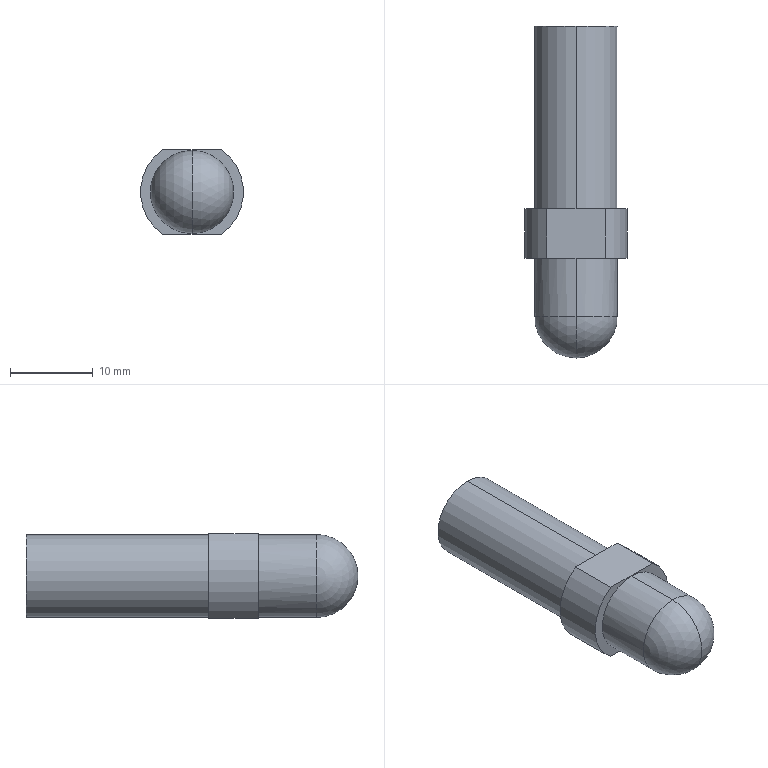Part | 1 solid | 13 faces | box 12.4 x 40 x 10.2 mm | volume 3201 mm3 | cylinder 6 | plane 5 | sphere 2 | commonest cylinder face diameters 10 x4 12.4 x2
STEP:
#1=CARTESIAN_POINT('',(0.,-12.,0.));
#2=VERTEX_POINT('',#1);
#3=CARTESIAN_POINT('',(0.,-7.,5.));
#4=VERTEX_POINT('',#3);
#5=CARTESIAN_POINT('',(0.,-7.,0.));
#6=DIRECTION('',(-1.,0.,0.));
#7=DIRECTION('',(0.,0.,1.));
#8=AXIS2_PLACEMENT_3D('',#5,#6,#7);
#9=CIRCLE('',#8,5.);
#10=EDGE_CURVE('',#2,#4,#9,.T.);
#11=ORIENTED_EDGE('',*,*,#10,.F.);
#12=CARTESIAN_POINT('',(0.,-7.,-5.));
#13=VERTEX_POINT('',#12);
#14=CARTESIAN_POINT('',(0.,-7.,0.));
#15=DIRECTION('',(1.,0.,0.));
#16=DIRECTION('',(0.,0.,-1.));
#17=AXIS2_PLACEMENT_3D('',#14,#15,#16);
#18=CIRCLE('',#17,5.);
#19=EDGE_CURVE('',#2,#13,#18,.T.);
#20=ORIENTED_EDGE('',*,*,#19,.T.);
#21=CARTESIAN_POINT('',(0.,-7.,0.));
#22=DIRECTION('',(0.,-1.,0.));
#23=DIRECTION('',(0.,0.,-1.));
#24=AXIS2_PLACEMENT_3D('',#21,#22,#23);
#25=CIRCLE('',#24,5.);
#26=EDGE_CURVE('',#13,#4,#25,.T.);
#27=ORIENTED_EDGE('',*,*,#26,.T.);
#28=EDGE_LOOP('',(#11,#20,#27));
#29=FACE_OUTER_BOUND('',#28,.T.);
#30=CARTESIAN_POINT('',(0.,-7.,0.));
#31=DIRECTION('',(1.,0.,0.));
#32=DIRECTION('',(0.,0.,1.));
#33=AXIS2_PLACEMENT_3D('',#30,#31,#32);
#34=SPHERICAL_SURFACE('',#33,5.);
#35=ADVANCED_FACE('',(#29),#34,.T.);
#36=ORIENTED_EDGE('',*,*,#26,.F.);
#37=CARTESIAN_POINT('',(0.,0.,-5.));
#38=VERTEX_POINT('',#37);
#39=CARTESIAN_POINT('',(0.,-7.,-5.));
#40=DIRECTION('',(0.,1.,0.));
#41=VECTOR('',#40,1000.);
#42=LINE('',#39,#41);
#43=EDGE_CURVE('',#13,#38,#42,.T.);
#44=ORIENTED_EDGE('',*,*,#43,.T.);
#45=CARTESIAN_POINT('',(0.,0.,5.));
#46=VERTEX_POINT('',#45);
#47=CARTESIAN_POINT('',(0.,0.,0.));
#48=DIRECTION('',(0.,-1.,0.));
#49=DIRECTION('',(0.,0.,1.));
#50=AXIS2_PLACEMENT_3D('',#47,#48,#49);
#51=CIRCLE('',#50,5.);
#52=EDGE_CURVE('',#38,#46,#51,.T.);
#53=ORIENTED_EDGE('',*,*,#52,.T.);
#54=CARTESIAN_POINT('',(0.,-7.,5.));
#55=DIRECTION('',(0.,1.,0.));
#56=VECTOR('',#55,1000.);
#57=LINE('',#54,#56);
#58=EDGE_CURVE('',#4,#46,#57,.T.);
#59=ORIENTED_EDGE('',*,*,#58,.F.);
#60=EDGE_LOOP('',(#36,#44,#53,#59));
#61=FACE_OUTER_BOUND('',#60,.T.);
#62=CARTESIAN_POINT('',(0.,-7.,0.));
#63=DIRECTION('',(0.,1.,0.));
#64=DIRECTION('',(0.,0.,1.));
#65=AXIS2_PLACEMENT_3D('',#62,#63,#64);
#66=CYLINDRICAL_SURFACE('',#65,5.);
#67=ADVANCED_FACE('',(#61),#66,.T.);
#68=CARTESIAN_POINT('',(0.,28.,5.));
#69=VERTEX_POINT('',#68);
#70=CARTESIAN_POINT('',(0.,28.,-5.));
#71=VERTEX_POINT('',#70);
#72=CARTESIAN_POINT('',(0.,28.,0.));
#73=DIRECTION('',(0.,1.,0.));
#74=DIRECTION('',(0.,0.,1.));
#75=AXIS2_PLACEMENT_3D('',#72,#73,#74);
#76=CIRCLE('',#75,5.);
#77=EDGE_CURVE('',#69,#71,#76,.T.);
#78=ORIENTED_EDGE('',*,*,#77,.F.);
#79=CARTESIAN_POINT('',(0.,6.,5.));
#80=VERTEX_POINT('',#79);
#81=CARTESIAN_POINT('',(0.,28.,5.));
#82=DIRECTION('',(0.,-1.,0.));
#83=VECTOR('',#82,1000.);
#84=LINE('',#81,#83);
#85=EDGE_CURVE('',#69,#80,#84,.T.);
#86=ORIENTED_EDGE('',*,*,#85,.T.);
#87=CARTESIAN_POINT('',(0.,6.,-5.));
#88=VERTEX_POINT('',#87);
#89=CARTESIAN_POINT('',(0.,6.,0.));
#90=DIRECTION('',(0.,1.,0.));
#91=DIRECTION('',(0.,0.,1.));
#92=AXIS2_PLACEMENT_3D('',#89,#90,#91);
#93=CIRCLE('',#92,5.);
#94=EDGE_CURVE('',#80,#88,#93,.T.);
#95=ORIENTED_EDGE('',*,*,#94,.T.);
#96=CARTESIAN_POINT('',(0.,28.,-5.));
#97=DIRECTION('',(0.,-1.,0.));
#98=VECTOR('',#97,1000.);
#99=LINE('',#96,#98);
#100=EDGE_CURVE('',#71,#88,#99,.T.);
#101=ORIENTED_EDGE('',*,*,#100,.F.);
#102=EDGE_LOOP('',(#78,#86,#95,#101));
#103=FACE_OUTER_BOUND('',#102,.T.);
#104=CARTESIAN_POINT('',(0.,28.,0.));
#105=DIRECTION('',(0.,-1.,0.));
#106=DIRECTION('',(0.,0.,-1.));
#107=AXIS2_PLACEMENT_3D('',#104,#105,#106);
#108=CYLINDRICAL_SURFACE('',#107,5.);
#109=ADVANCED_FACE('',(#103),#108,.T.);
#110=CARTESIAN_POINT('',(-3.526,6.,-5.1));
#111=VERTEX_POINT('',#110);
#112=CARTESIAN_POINT('',(-3.526,6.,5.1));
#113=VERTEX_POINT('',#112);
#114=CARTESIAN_POINT('',(0.,6.,0.));
#115=DIRECTION('',(0.,1.,0.));
#116=DIRECTION('',(0.,0.,1.));
#117=AXIS2_PLACEMENT_3D('',#114,#115,#116);
#118=CIRCLE('',#117,6.2);
#119=EDGE_CURVE('',#111,#113,#118,.T.);
#120=ORIENTED_EDGE('',*,*,#119,.F.);
#121=CARTESIAN_POINT('',(-3.526,0.,-5.1));
#122=VERTEX_POINT('',#121);
#123=CARTESIAN_POINT('',(-3.526,6.,-5.1));
#124=DIRECTION('',(0.,-1.,0.));
#125=VECTOR('',#124,1000.);
#126=LINE('',#123,#125);
#127=EDGE_CURVE('',#111,#122,#126,.T.);
#128=ORIENTED_EDGE('',*,*,#127,.T.);
#129=CARTESIAN_POINT('',(-3.526,0.,5.1));
#130=VERTEX_POINT('',#129);
#131=CARTESIAN_POINT('',(0.,0.,0.));
#132=DIRECTION('',(0.,1.,0.));
#133=DIRECTION('',(0.,0.,1.));
#134=AXIS2_PLACEMENT_3D('',#131,#132,#133);
#135=CIRCLE('',#134,6.2);
#136=EDGE_CURVE('',#122,#130,#135,.T.);
#137=ORIENTED_EDGE('',*,*,#136,.T.);
#138=CARTESIAN_POINT('',(-3.526,6.,5.1));
#139=DIRECTION('',(0.,1.,0.));
#140=VECTOR('',#139,1000.);
#141=LINE('',#138,#140);
#142=EDGE_CURVE('',#130,#113,#141,.T.);
#143=ORIENTED_EDGE('',*,*,#142,.T.);
#144=EDGE_LOOP('',(#120,#128,#137,#143));
#145=FACE_OUTER_BOUND('',#144,.T.);
#146=CARTESIAN_POINT('',(0.,6.,0.));
#147=DIRECTION('',(0.,-1.,0.));
#148=DIRECTION('',(0.,0.,-1.));
#149=AXIS2_PLACEMENT_3D('',#146,#147,#148);
#150=CYLINDRICAL_SURFACE('',#149,6.2);
#151=ADVANCED_FACE('',(#145),#150,.T.);
#152=CARTESIAN_POINT('',(3.526,0.,5.1));
#153=VERTEX_POINT('',#152);
#154=CARTESIAN_POINT('',(3.526,0.,-5.1));
#155=VERTEX_POINT('',#154);
#156=CARTESIAN_POINT('',(0.,0.,0.));
#157=DIRECTION('',(0.,1.,0.));
#158=DIRECTION('',(0.,0.,1.));
#159=AXIS2_PLACEMENT_3D('',#156,#157,#158);
#160=CIRCLE('',#159,6.2);
#161=EDGE_CURVE('',#153,#155,#160,.T.);
#162=ORIENTED_EDGE('',*,*,#161,.T.);
#163=CARTESIAN_POINT('',(3.526,6.,-5.1));
#164=VERTEX_POINT('',#163);
#165=CARTESIAN_POINT('',(3.526,6.,-5.1));
#166=DIRECTION('',(0.,1.,0.));
#167=VECTOR('',#166,1000.);
#168=LINE('',#165,#167);
#169=EDGE_CURVE('',#155,#164,#168,.T.);
#170=ORIENTED_EDGE('',*,*,#169,.T.);
#171=CARTESIAN_POINT('',(3.526,6.,5.1));
#172=VERTEX_POINT('',#171);
#173=CARTESIAN_POINT('',(0.,6.,0.));
#174=DIRECTION('',(0.,1.,0.));
#175=DIRECTION('',(0.,0.,1.));
#176=AXIS2_PLACEMENT_3D('',#173,#174,#175);
#177=CIRCLE('',#176,6.2);
#178=EDGE_CURVE('',#172,#164,#177,.T.);
#179=ORIENTED_EDGE('',*,*,#178,.F.);
#180=CARTESIAN_POINT('',(3.526,6.,5.1));
#181=DIRECTION('',(0.,-1.,0.));
#182=VECTOR('',#181,1000.);
#183=LINE('',#180,#182);
#184=EDGE_CURVE('',#172,#153,#183,.T.);
#185=ORIENTED_EDGE('',*,*,#184,.T.);
#186=EDGE_LOOP('',(#162,#170,#179,#185));
#187=FACE_OUTER_BOUND('',#186,.T.);
#188=CARTESIAN_POINT('',(0.,6.,0.));
#189=DIRECTION('',(0.,-1.,0.));
#190=DIRECTION('',(0.,0.,-1.));
#191=AXIS2_PLACEMENT_3D('',#188,#189,#190);
#192=CYLINDRICAL_SURFACE('',#191,6.2);
#193=ADVANCED_FACE('',(#187),#192,.T.);
#194=CARTESIAN_POINT('',(-6.5,6.,-5.1));
#195=DIRECTION('',(-1.,0.,0.));
#196=VECTOR('',#195,1000.);
#197=LINE('',#194,#196);
#198=EDGE_CURVE('',#164,#111,#197,.T.);
#199=ORIENTED_EDGE('',*,*,#198,.T.);
#200=ORIENTED_EDGE('',*,*,#119,.T.);
#201=CARTESIAN_POINT('',(-6.5,6.,5.1));
#202=DIRECTION('',(1.,0.,0.));
#203=VECTOR('',#202,1000.);
#204=LINE('',#201,#203);
#205=EDGE_CURVE('',#113,#172,#204,.T.);
#206=ORIENTED_EDGE('',*,*,#205,.T.);
#207=ORIENTED_EDGE('',*,*,#178,.T.);
#208=EDGE_LOOP('',(#199,#200,#206,#207));
#209=FACE_OUTER_BOUND('',#208,.T.);
#210=CARTESIAN_POINT('',(0.,6.,0.));
#211=DIRECTION('',(0.,1.,0.));
#212=DIRECTION('',(0.,0.,1.));
#213=AXIS2_PLACEMENT_3D('',#210,#211,#212);
#214=CIRCLE('',#213,5.);
#215=EDGE_CURVE('',#88,#80,#214,.T.);
#216=ORIENTED_EDGE('',*,*,#215,.F.);
#217=ORIENTED_EDGE('',*,*,#94,.F.);
#218=EDGE_LOOP('',(#216,#217));
#219=FACE_BOUND('',#218,.T.);
#220=CARTESIAN_POINT('',(0.,6.,0.));
#221=DIRECTION('',(0.,1.,0.));
#222=DIRECTION('',(1.,0.,0.));
#223=AXIS2_PLACEMENT_3D('',#220,#221,#222);
#224=PLANE('',#223);
#225=ADVANCED_FACE('',(#209,#219),#224,.T.);
#226=ORIENTED_EDGE('',*,*,#136,.F.);
#227=CARTESIAN_POINT('',(0.,0.,-5.1));
#228=DIRECTION('',(1.,0.,0.));
#229=VECTOR('',#228,1000.);
#230=LINE('',#227,#229);
#231=EDGE_CURVE('',#122,#155,#230,.T.);
#232=ORIENTED_EDGE('',*,*,#231,.T.);
#233=ORIENTED_EDGE('',*,*,#161,.F.);
#234=CARTESIAN_POINT('',(0.,0.,5.1));
#235=DIRECTION('',(-1.,0.,0.));
#236=VECTOR('',#235,1000.);
#237=LINE('',#234,#236);
#238=EDGE_CURVE('',#153,#130,#237,.T.);
#239=ORIENTED_EDGE('',*,*,#238,.T.);
#240=EDGE_LOOP('',(#226,#232,#233,#239));
#241=FACE_OUTER_BOUND('',#240,.T.);
#242=CARTESIAN_POINT('',(0.,0.,0.));
#243=DIRECTION('',(0.,-1.,0.));
#244=DIRECTION('',(0.,0.,1.));
#245=AXIS2_PLACEMENT_3D('',#242,#243,#244);
#246=CIRCLE('',#245,5.);
#247=EDGE_CURVE('',#46,#38,#246,.T.);
#248=ORIENTED_EDGE('',*,*,#247,.F.);
#249=ORIENTED_EDGE('',*,*,#52,.F.);
#250=EDGE_LOOP('',(#248,#249));
#251=FACE_BOUND('',#250,.T.);
#252=CARTESIAN_POINT('',(0.,0.,0.));
#253=DIRECTION('',(0.,1.,0.));
#254=DIRECTION('',(1.,0.,0.));
#255=AXIS2_PLACEMENT_3D('',#252,#253,#254);
#256=PLANE('',#255);
#257=ADVANCED_FACE('',(#241,#251),#256,.F.);
#258=ORIENTED_EDGE('',*,*,#205,.F.);
#259=ORIENTED_EDGE('',*,*,#142,.F.);
#260=ORIENTED_EDGE('',*,*,#238,.F.);
#261=ORIENTED_EDGE('',*,*,#184,.F.);
#262=EDGE_LOOP('',(#258,#259,#260,#261));
#263=FACE_OUTER_BOUND('',#262,.T.);
#264=CARTESIAN_POINT('',(-6.5,6.,5.1));
#265=DIRECTION('',(0.,0.,-1.));
#266=DIRECTION('',(0.,-1.,0.));
#267=AXIS2_PLACEMENT_3D('',#264,#265,#266);
#268=PLANE('',#267);
#269=ADVANCED_FACE('',(#263),#268,.F.);
#270=ORIENTED_EDGE('',*,*,#198,.F.);
#271=ORIENTED_EDGE('',*,*,#169,.F.);
#272=ORIENTED_EDGE('',*,*,#231,.F.);
#273=ORIENTED_EDGE('',*,*,#127,.F.);
#274=EDGE_LOOP('',(#270,#271,#272,#273));
#275=FACE_OUTER_BOUND('',#274,.T.);
#276=CARTESIAN_POINT('',(-6.5,6.,-5.1));
#277=DIRECTION('',(0.,0.,1.));
#278=DIRECTION('',(1.,0.,0.));
#279=AXIS2_PLACEMENT_3D('',#276,#277,#278);
#280=PLANE('',#279);
#281=ADVANCED_FACE('',(#275),#280,.F.);
#282=ORIENTED_EDGE('',*,*,#85,.F.);
#283=CARTESIAN_POINT('',(0.,28.,0.));
#284=DIRECTION('',(0.,1.,0.));
#285=DIRECTION('',(0.,0.,1.));
#286=AXIS2_PLACEMENT_3D('',#283,#284,#285);
#287=CIRCLE('',#286,5.);
#288=EDGE_CURVE('',#71,#69,#287,.T.);
#289=ORIENTED_EDGE('',*,*,#288,.F.);
#290=ORIENTED_EDGE('',*,*,#100,.T.);
#291=ORIENTED_EDGE('',*,*,#215,.T.);
#292=EDGE_LOOP('',(#282,#289,#290,#291));
#293=FACE_OUTER_BOUND('',#292,.T.);
#294=CARTESIAN_POINT('',(0.,28.,0.));
#295=DIRECTION('',(0.,-1.,0.));
#296=DIRECTION('',(0.,0.,-1.));
#297=AXIS2_PLACEMENT_3D('',#294,#295,#296);
#298=CYLINDRICAL_SURFACE('',#297,5.);
#299=ADVANCED_FACE('',(#293),#298,.T.);
#300=ORIENTED_EDGE('',*,*,#288,.T.);
#301=ORIENTED_EDGE('',*,*,#77,.T.);
#302=EDGE_LOOP('',(#300,#301));
#303=FACE_OUTER_BOUND('',#302,.T.);
#304=CARTESIAN_POINT('',(0.,28.,0.));
#305=DIRECTION('',(0.,1.,0.));
#306=DIRECTION('',(1.,0.,0.));
#307=AXIS2_PLACEMENT_3D('',#304,#305,#306);
#308=PLANE('',#307);
#309=ADVANCED_FACE('',(#303),#308,.T.);
#310=ORIENTED_EDGE('',*,*,#43,.F.);
#311=CARTESIAN_POINT('',(0.,-7.,0.));
#312=DIRECTION('',(0.,-1.,0.));
#313=DIRECTION('',(0.,0.,-1.));
#314=AXIS2_PLACEMENT_3D('',#311,#312,#313);
#315=CIRCLE('',#314,5.);
#316=EDGE_CURVE('',#4,#13,#315,.T.);
#317=ORIENTED_EDGE('',*,*,#316,.F.);
#318=ORIENTED_EDGE('',*,*,#58,.T.);
#319=ORIENTED_EDGE('',*,*,#247,.T.);
#320=EDGE_LOOP('',(#310,#317,#318,#319));
#321=FACE_OUTER_BOUND('',#320,.T.);
#322=CARTESIAN_POINT('',(0.,-7.,0.));
#323=DIRECTION('',(0.,1.,0.));
#324=DIRECTION('',(0.,0.,1.));
#325=AXIS2_PLACEMENT_3D('',#322,#323,#324);
#326=CYLINDRICAL_SURFACE('',#325,5.);
#327=ADVANCED_FACE('',(#321),#326,.T.);
#328=ORIENTED_EDGE('',*,*,#19,.F.);
#329=ORIENTED_EDGE('',*,*,#10,.T.);
#330=ORIENTED_EDGE('',*,*,#316,.T.);
#331=EDGE_LOOP('',(#328,#329,#330));
#332=FACE_OUTER_BOUND('',#331,.T.);
#333=CARTESIAN_POINT('',(0.,-7.,0.));
#334=DIRECTION('',(1.,0.,0.));
#335=DIRECTION('',(0.,0.,1.));
#336=AXIS2_PLACEMENT_3D('',#333,#334,#335);
#337=SPHERICAL_SURFACE('',#336,5.);
#338=ADVANCED_FACE('',(#332),#337,.T.);
#339=CLOSED_SHELL('',(#35,#67,#109,#151,#193,#225,#257,#269,#281,#299,#309,#327,#338));
#340=MANIFOLD_SOLID_BREP('',#339);
#341=CARTESIAN_POINT('',(0.,0.,0.));
#342=DIRECTION('',(0.,0.,1.));
#343=DIRECTION('',(1.,0.,0.));
#344=AXIS2_PLACEMENT_3D('',#341,#342,#343);
#345=(LENGTH_UNIT()NAMED_UNIT(*)SI_UNIT(.MILLI.,.METRE.));
#346=UNCERTAINTY_MEASURE_WITH_UNIT(LENGTH_MEASURE(0.00001),#345,'','');
#347=(NAMED_UNIT(*)PLANE_ANGLE_UNIT()SI_UNIT($,.RADIAN.));
#348=(NAMED_UNIT(*)SI_UNIT($,.STERADIAN.)SOLID_ANGLE_UNIT());
#349=(GEOMETRIC_REPRESENTATION_CONTEXT(3)GLOBAL_UNCERTAINTY_ASSIGNED_CONTEXT((#346))GLOBAL_UNIT_ASSIGNED_CONTEXT((#345,#347,#348))REPRESENTATION_CONTEXT('',''));
#350=ADVANCED_BREP_SHAPE_REPRESENTATION('',(#340,#344),#349);